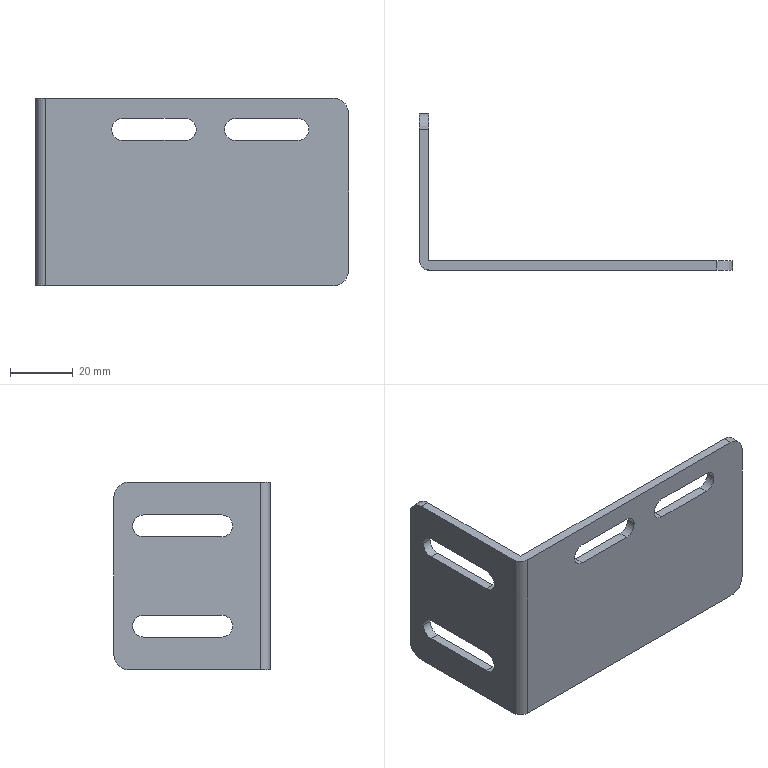Part | STEP file | X Travel Bracket 2 | 1 solid | 32 faces | box 100 x 50 x 60 mm | volume 23920 mm3 | cylinder 16 | plane 16 | commonest cylinder face diameters 7 x10 10 x4 0.2 x1 6.2 x1
STEP:
#1=CARTESIAN_POINT('',(-18.962,-0.4258,49.5));
#2=VERTEX_POINT('',#1);
#3=CARTESIAN_POINT('',(-18.962,3.074,46.));
#4=VERTEX_POINT('',#3);
#5=CARTESIAN_POINT('',(-18.962,-0.4258,46.));
#6=DIRECTION('',(-1.,0.,0.));
#7=DIRECTION('',(0.,1.,0.));
#8=AXIS2_PLACEMENT_3D('',#5,#6,#7);
#9=CIRCLE('',#8,3.5);
#10=EDGE_CURVE('',#2,#4,#9,.T.);
#11=ORIENTED_EDGE('',*,*,#10,.T.);
#12=CARTESIAN_POINT('',(-15.962,3.074,46.));
#13=VERTEX_POINT('',#12);
#14=CARTESIAN_POINT('',(-25.962,3.074,46.));
#15=DIRECTION('',(1.,0.,0.));
#16=VECTOR('',#15,1000.);
#17=LINE('',#14,#16);
#18=EDGE_CURVE('',#4,#13,#17,.T.);
#19=ORIENTED_EDGE('',*,*,#18,.T.);
#20=CARTESIAN_POINT('',(-15.962,-0.4258,49.5));
#21=VERTEX_POINT('',#20);
#22=CARTESIAN_POINT('',(-15.962,-0.4258,46.));
#23=DIRECTION('',(-1.,0.,0.));
#24=DIRECTION('',(0.,1.,0.));
#25=AXIS2_PLACEMENT_3D('',#22,#23,#24);
#26=CIRCLE('',#25,3.5);
#27=EDGE_CURVE('',#21,#13,#26,.T.);
#28=ORIENTED_EDGE('',*,*,#27,.F.);
#29=CARTESIAN_POINT('',(-25.962,-0.4258,49.5));
#30=DIRECTION('',(1.,0.,0.));
#31=VECTOR('',#30,1000.);
#32=LINE('',#29,#31);
#33=EDGE_CURVE('',#2,#21,#32,.T.);
#34=ORIENTED_EDGE('',*,*,#33,.F.);
#35=EDGE_LOOP('',(#11,#19,#28,#34));
#36=FACE_OUTER_BOUND('',#35,.T.);
#37=CARTESIAN_POINT('',(-25.962,-0.4258,46.));
#38=DIRECTION('',(1.,0.,0.));
#39=DIRECTION('',(0.,1.,0.));
#40=AXIS2_PLACEMENT_3D('',#37,#38,#39);
#41=CYLINDRICAL_SURFACE('',#40,3.5);
#42=ADVANCED_FACE('',(#36),#41,.F.);
#43=CARTESIAN_POINT('',(-18.962,-0.4258,17.5));
#44=VERTEX_POINT('',#43);
#45=CARTESIAN_POINT('',(-18.962,3.074,14.));
#46=VERTEX_POINT('',#45);
#47=CARTESIAN_POINT('',(-18.962,-0.4258,14.));
#48=DIRECTION('',(-1.,0.,0.));
#49=DIRECTION('',(0.,1.,0.));
#50=AXIS2_PLACEMENT_3D('',#47,#48,#49);
#51=CIRCLE('',#50,3.5);
#52=EDGE_CURVE('',#44,#46,#51,.T.);
#53=ORIENTED_EDGE('',*,*,#52,.T.);
#54=CARTESIAN_POINT('',(-15.962,3.074,14.));
#55=VERTEX_POINT('',#54);
#56=CARTESIAN_POINT('',(-25.962,3.074,14.));
#57=DIRECTION('',(1.,0.,0.));
#58=VECTOR('',#57,1000.);
#59=LINE('',#56,#58);
#60=EDGE_CURVE('',#46,#55,#59,.T.);
#61=ORIENTED_EDGE('',*,*,#60,.T.);
#62=CARTESIAN_POINT('',(-15.962,-0.4258,17.5));
#63=VERTEX_POINT('',#62);
#64=CARTESIAN_POINT('',(-15.962,-0.4258,14.));
#65=DIRECTION('',(-1.,0.,0.));
#66=DIRECTION('',(0.,1.,0.));
#67=AXIS2_PLACEMENT_3D('',#64,#65,#66);
#68=CIRCLE('',#67,3.5);
#69=EDGE_CURVE('',#63,#55,#68,.T.);
#70=ORIENTED_EDGE('',*,*,#69,.F.);
#71=CARTESIAN_POINT('',(-25.962,-0.4258,17.5));
#72=DIRECTION('',(1.,0.,0.));
#73=VECTOR('',#72,1000.);
#74=LINE('',#71,#73);
#75=EDGE_CURVE('',#44,#63,#74,.T.);
#76=ORIENTED_EDGE('',*,*,#75,.F.);
#77=EDGE_LOOP('',(#53,#61,#70,#76));
#78=FACE_OUTER_BOUND('',#77,.T.);
#79=CARTESIAN_POINT('',(-25.962,-0.4258,14.));
#80=DIRECTION('',(1.,0.,0.));
#81=DIRECTION('',(0.,1.,0.));
#82=AXIS2_PLACEMENT_3D('',#79,#80,#81);
#83=CYLINDRICAL_SURFACE('',#82,3.5);
#84=ADVANCED_FACE('',(#78),#83,.F.);
#85=CARTESIAN_POINT('',(81.038,-40.926,5.));
#86=VERTEX_POINT('',#85);
#87=CARTESIAN_POINT('',(76.038,-40.926,0.));
#88=VERTEX_POINT('',#87);
#89=CARTESIAN_POINT('',(76.038,-40.926,5.));
#90=DIRECTION('',(0.,1.,0.));
#91=DIRECTION('',(0.,0.,-1.));
#92=AXIS2_PLACEMENT_3D('',#89,#90,#91);
#93=CIRCLE('',#92,5.);
#94=EDGE_CURVE('',#86,#88,#93,.T.);
#95=ORIENTED_EDGE('',*,*,#94,.F.);
#96=CARTESIAN_POINT('',(81.038,-40.926,55.));
#97=VERTEX_POINT('',#96);
#98=CARTESIAN_POINT('',(81.038,-40.926,60.));
#99=DIRECTION('',(0.,0.,-1.));
#100=VECTOR('',#99,1000.);
#101=LINE('',#98,#100);
#102=EDGE_CURVE('',#97,#86,#101,.T.);
#103=ORIENTED_EDGE('',*,*,#102,.F.);
#104=CARTESIAN_POINT('',(76.038,-40.926,60.));
#105=VERTEX_POINT('',#104);
#106=CARTESIAN_POINT('',(76.038,-40.926,55.));
#107=DIRECTION('',(0.,1.,0.));
#108=DIRECTION('',(0.,0.,-1.));
#109=AXIS2_PLACEMENT_3D('',#106,#107,#108);
#110=CIRCLE('',#109,5.);
#111=EDGE_CURVE('',#105,#97,#110,.T.);
#112=ORIENTED_EDGE('',*,*,#111,.F.);
#113=CARTESIAN_POINT('',(-15.862,-40.926,60.));
#114=VERTEX_POINT('',#113);
#115=CARTESIAN_POINT('',(-18.962,-40.926,60.));
#116=DIRECTION('',(1.,0.,0.));
#117=VECTOR('',#116,1000.);
#118=LINE('',#115,#117);
#119=EDGE_CURVE('',#114,#105,#118,.T.);
#120=ORIENTED_EDGE('',*,*,#119,.F.);
#121=CARTESIAN_POINT('',(-15.862,-40.926,0.));
#122=VERTEX_POINT('',#121);
#123=CARTESIAN_POINT('',(-15.862,-40.926,60.));
#124=DIRECTION('',(0.,0.,1.));
#125=VECTOR('',#124,1000.);
#126=LINE('',#123,#125);
#127=EDGE_CURVE('',#122,#114,#126,.T.);
#128=ORIENTED_EDGE('',*,*,#127,.F.);
#129=CARTESIAN_POINT('',(-18.962,-40.926,0.));
#130=DIRECTION('',(-1.,0.,0.));
#131=VECTOR('',#130,1000.);
#132=LINE('',#129,#131);
#133=EDGE_CURVE('',#88,#122,#132,.T.);
#134=ORIENTED_EDGE('',*,*,#133,.F.);
#135=EDGE_LOOP('',(#95,#103,#112,#120,#128,#134));
#136=FACE_OUTER_BOUND('',#135,.T.);
#137=CARTESIAN_POINT('',(8.866,-40.926,53.5));
#138=VERTEX_POINT('',#137);
#139=CARTESIAN_POINT('',(8.866,-40.926,46.5));
#140=VERTEX_POINT('',#139);
#141=CARTESIAN_POINT('',(8.866,-40.926,50.));
#142=DIRECTION('',(0.,-1.,0.));
#143=DIRECTION('',(0.,0.,1.));
#144=AXIS2_PLACEMENT_3D('',#141,#142,#143);
#145=CIRCLE('',#144,3.5);
#146=EDGE_CURVE('',#138,#140,#145,.T.);
#147=ORIENTED_EDGE('',*,*,#146,.F.);
#148=CARTESIAN_POINT('',(28.866,-40.926,53.5));
#149=VERTEX_POINT('',#148);
#150=CARTESIAN_POINT('',(-18.962,-40.926,53.5));
#151=DIRECTION('',(-1.,0.,0.));
#152=VECTOR('',#151,1000.);
#153=LINE('',#150,#152);
#154=EDGE_CURVE('',#149,#138,#153,.T.);
#155=ORIENTED_EDGE('',*,*,#154,.F.);
#156=CARTESIAN_POINT('',(28.866,-40.926,46.5));
#157=VERTEX_POINT('',#156);
#158=CARTESIAN_POINT('',(28.866,-40.926,50.));
#159=DIRECTION('',(0.,-1.,0.));
#160=DIRECTION('',(0.,0.,1.));
#161=AXIS2_PLACEMENT_3D('',#158,#159,#160);
#162=CIRCLE('',#161,3.5);
#163=EDGE_CURVE('',#157,#149,#162,.T.);
#164=ORIENTED_EDGE('',*,*,#163,.F.);
#165=CARTESIAN_POINT('',(-18.962,-40.926,46.5));
#166=DIRECTION('',(1.,0.,0.));
#167=VECTOR('',#166,1000.);
#168=LINE('',#165,#167);
#169=EDGE_CURVE('',#140,#157,#168,.T.);
#170=ORIENTED_EDGE('',*,*,#169,.F.);
#171=EDGE_LOOP('',(#147,#155,#164,#170));
#172=FACE_BOUND('',#171,.T.);
#173=CARTESIAN_POINT('',(44.866,-40.926,53.5));
#174=VERTEX_POINT('',#173);
#175=CARTESIAN_POINT('',(44.866,-40.926,46.5));
#176=VERTEX_POINT('',#175);
#177=CARTESIAN_POINT('',(44.866,-40.926,50.));
#178=DIRECTION('',(0.,-1.,0.));
#179=DIRECTION('',(0.,0.,1.));
#180=AXIS2_PLACEMENT_3D('',#177,#178,#179);
#181=CIRCLE('',#180,3.5);
#182=EDGE_CURVE('',#174,#176,#181,.T.);
#183=ORIENTED_EDGE('',*,*,#182,.F.);
#184=CARTESIAN_POINT('',(64.866,-40.926,53.5));
#185=VERTEX_POINT('',#184);
#186=CARTESIAN_POINT('',(-18.962,-40.926,53.5));
#187=DIRECTION('',(-1.,0.,0.));
#188=VECTOR('',#187,1000.);
#189=LINE('',#186,#188);
#190=EDGE_CURVE('',#185,#174,#189,.T.);
#191=ORIENTED_EDGE('',*,*,#190,.F.);
#192=CARTESIAN_POINT('',(64.866,-40.926,46.5));
#193=VERTEX_POINT('',#192);
#194=CARTESIAN_POINT('',(64.866,-40.926,50.));
#195=DIRECTION('',(0.,-1.,0.));
#196=DIRECTION('',(0.,0.,1.));
#197=AXIS2_PLACEMENT_3D('',#194,#195,#196);
#198=CIRCLE('',#197,3.5);
#199=EDGE_CURVE('',#193,#185,#198,.T.);
#200=ORIENTED_EDGE('',*,*,#199,.F.);
#201=CARTESIAN_POINT('',(-18.962,-40.926,46.5));
#202=DIRECTION('',(1.,0.,0.));
#203=VECTOR('',#202,1000.);
#204=LINE('',#201,#203);
#205=EDGE_CURVE('',#176,#193,#204,.T.);
#206=ORIENTED_EDGE('',*,*,#205,.F.);
#207=EDGE_LOOP('',(#183,#191,#200,#206));
#208=FACE_BOUND('',#207,.T.);
#209=CARTESIAN_POINT('',(-18.962,-40.926,60.));
#210=DIRECTION('',(0.,1.,0.));
#211=DIRECTION('',(0.,0.,1.));
#212=AXIS2_PLACEMENT_3D('',#209,#210,#211);
#213=PLANE('',#212);
#214=ADVANCED_FACE('',(#136,#172,#208),#213,.F.);
#215=ORIENTED_EDGE('',*,*,#133,.T.);
#216=CARTESIAN_POINT('',(-18.962,-37.826,0.));
#217=VERTEX_POINT('',#216);
#218=CARTESIAN_POINT('',(-15.862,-37.826,0.));
#219=DIRECTION('',(0.,0.,1.));
#220=DIRECTION('',(-1.,0.,0.));
#221=AXIS2_PLACEMENT_3D('',#218,#219,#220);
#222=CIRCLE('',#221,3.1);
#223=EDGE_CURVE('',#217,#122,#222,.T.);
#224=ORIENTED_EDGE('',*,*,#223,.F.);
#225=CARTESIAN_POINT('',(-18.962,4.074,0.));
#226=VERTEX_POINT('',#225);
#227=CARTESIAN_POINT('',(-18.962,9.074,0.));
#228=DIRECTION('',(0.,1.,0.));
#229=VECTOR('',#228,1000.);
#230=LINE('',#227,#229);
#231=EDGE_CURVE('',#217,#226,#230,.T.);
#232=ORIENTED_EDGE('',*,*,#231,.T.);
#233=CARTESIAN_POINT('',(-15.962,4.074,0.));
#234=VERTEX_POINT('',#233);
#235=CARTESIAN_POINT('',(-15.862,4.074,0.));
#236=DIRECTION('',(-1.,0.,0.));
#237=VECTOR('',#236,1000.);
#238=LINE('',#235,#237);
#239=EDGE_CURVE('',#234,#226,#238,.T.);
#240=ORIENTED_EDGE('',*,*,#239,.F.);
#241=CARTESIAN_POINT('',(-15.962,-37.826,0.));
#242=VERTEX_POINT('',#241);
#243=CARTESIAN_POINT('',(-15.962,-37.826,0.));
#244=DIRECTION('',(0.,1.,0.));
#245=VECTOR('',#244,1000.);
#246=LINE('',#243,#245);
#247=EDGE_CURVE('',#242,#234,#246,.T.);
#248=ORIENTED_EDGE('',*,*,#247,.F.);
#249=CARTESIAN_POINT('',(-15.862,-37.926,0.));
#250=VERTEX_POINT('',#249);
#251=CARTESIAN_POINT('',(-15.862,-37.826,0.));
#252=DIRECTION('',(0.,0.,1.));
#253=DIRECTION('',(-1.,0.,0.));
#254=AXIS2_PLACEMENT_3D('',#251,#252,#253);
#255=CIRCLE('',#254,0.1);
#256=EDGE_CURVE('',#242,#250,#255,.T.);
#257=ORIENTED_EDGE('',*,*,#256,.T.);
#258=CARTESIAN_POINT('',(76.038,-37.926,0.));
#259=VERTEX_POINT('',#258);
#260=CARTESIAN_POINT('',(-15.962,-37.926,0.));
#261=DIRECTION('',(1.,0.,0.));
#262=VECTOR('',#261,1000.);
#263=LINE('',#260,#262);
#264=EDGE_CURVE('',#250,#259,#263,.T.);
#265=ORIENTED_EDGE('',*,*,#264,.T.);
#266=CARTESIAN_POINT('',(76.038,-37.826,0.));
#267=DIRECTION('',(0.,-1.,0.));
#268=VECTOR('',#267,1000.);
#269=LINE('',#266,#268);
#270=EDGE_CURVE('',#259,#88,#269,.T.);
#271=ORIENTED_EDGE('',*,*,#270,.T.);
#272=EDGE_LOOP('',(#215,#224,#232,#240,#248,#257,#265,#271));
#273=FACE_OUTER_BOUND('',#272,.T.);
#274=CARTESIAN_POINT('',(-15.962,-37.826,0.));
#275=DIRECTION('',(0.,0.,-1.));
#276=DIRECTION('',(-1.,0.,0.));
#277=AXIS2_PLACEMENT_3D('',#274,#275,#276);
#278=PLANE('',#277);
#279=ADVANCED_FACE('',(#273),#278,.T.);
#280=ORIENTED_EDGE('',*,*,#94,.T.);
#281=ORIENTED_EDGE('',*,*,#270,.F.);
#282=CARTESIAN_POINT('',(81.038,-37.926,5.));
#283=VERTEX_POINT('',#282);
#284=CARTESIAN_POINT('',(76.038,-37.926,5.));
#285=DIRECTION('',(0.,-1.,0.));
#286=DIRECTION('',(0.,0.,-1.));
#287=AXIS2_PLACEMENT_3D('',#284,#285,#286);
#288=CIRCLE('',#287,5.);
#289=EDGE_CURVE('',#259,#283,#288,.T.);
#290=ORIENTED_EDGE('',*,*,#289,.T.);
#291=CARTESIAN_POINT('',(81.038,-37.826,5.));
#292=DIRECTION('',(0.,-1.,0.));
#293=VECTOR('',#292,1000.);
#294=LINE('',#291,#293);
#295=EDGE_CURVE('',#283,#86,#294,.T.);
#296=ORIENTED_EDGE('',*,*,#295,.T.);
#297=EDGE_LOOP('',(#280,#281,#290,#296));
#298=FACE_OUTER_BOUND('',#297,.T.);
#299=CARTESIAN_POINT('',(76.038,-37.826,5.));
#300=DIRECTION('',(0.,-1.,0.));
#301=DIRECTION('',(0.,0.,-1.));
#302=AXIS2_PLACEMENT_3D('',#299,#300,#301);
#303=CYLINDRICAL_SURFACE('',#302,5.);
#304=ADVANCED_FACE('',(#298),#303,.T.);
#305=CARTESIAN_POINT('',(81.038,-37.926,55.));
#306=VERTEX_POINT('',#305);
#307=CARTESIAN_POINT('',(81.038,-37.926,60.));
#308=DIRECTION('',(0.,0.,1.));
#309=VECTOR('',#308,1000.);
#310=LINE('',#307,#309);
#311=EDGE_CURVE('',#283,#306,#310,.T.);
#312=ORIENTED_EDGE('',*,*,#311,.T.);
#313=CARTESIAN_POINT('',(81.038,-37.926,55.));
#314=DIRECTION('',(0.,-1.,0.));
#315=VECTOR('',#314,1000.);
#316=LINE('',#313,#315);
#317=EDGE_CURVE('',#306,#97,#316,.T.);
#318=ORIENTED_EDGE('',*,*,#317,.T.);
#319=ORIENTED_EDGE('',*,*,#102,.T.);
#320=ORIENTED_EDGE('',*,*,#295,.F.);
#321=EDGE_LOOP('',(#312,#318,#319,#320));
#322=FACE_OUTER_BOUND('',#321,.T.);
#323=CARTESIAN_POINT('',(81.038,-37.926,60.));
#324=DIRECTION('',(1.,0.,0.));
#325=DIRECTION('',(0.,0.,-1.));
#326=AXIS2_PLACEMENT_3D('',#323,#324,#325);
#327=PLANE('',#326);
#328=ADVANCED_FACE('',(#322),#327,.T.);
#329=ORIENTED_EDGE('',*,*,#111,.T.);
#330=ORIENTED_EDGE('',*,*,#317,.F.);
#331=CARTESIAN_POINT('',(76.038,-37.926,60.));
#332=VERTEX_POINT('',#331);
#333=CARTESIAN_POINT('',(76.038,-37.926,55.));
#334=DIRECTION('',(0.,-1.,0.));
#335=DIRECTION('',(0.,0.,-1.));
#336=AXIS2_PLACEMENT_3D('',#333,#334,#335);
#337=CIRCLE('',#336,5.);
#338=EDGE_CURVE('',#306,#332,#337,.T.);
#339=ORIENTED_EDGE('',*,*,#338,.T.);
#340=CARTESIAN_POINT('',(76.038,-37.926,60.));
#341=DIRECTION('',(0.,-1.,0.));
#342=VECTOR('',#341,1000.);
#343=LINE('',#340,#342);
#344=EDGE_CURVE('',#332,#105,#343,.T.);
#345=ORIENTED_EDGE('',*,*,#344,.T.);
#346=EDGE_LOOP('',(#329,#330,#339,#345));
#347=FACE_OUTER_BOUND('',#346,.T.);
#348=CARTESIAN_POINT('',(76.038,-37.926,55.));
#349=DIRECTION('',(0.,-1.,0.));
#350=DIRECTION('',(0.,0.,-1.));
#351=AXIS2_PLACEMENT_3D('',#348,#349,#350);
#352=CYLINDRICAL_SURFACE('',#351,5.);
#353=ADVANCED_FACE('',(#347),#352,.T.);
#354=CARTESIAN_POINT('',(-15.862,-37.926,60.));
#355=VERTEX_POINT('',#354);
#356=CARTESIAN_POINT('',(-15.862,-37.926,60.));
#357=DIRECTION('',(-1.,0.,0.));
#358=VECTOR('',#357,1000.);
#359=LINE('',#356,#358);
#360=EDGE_CURVE('',#332,#355,#359,.T.);
#361=ORIENTED_EDGE('',*,*,#360,.T.);
#362=CARTESIAN_POINT('',(-15.962,-37.826,60.));
#363=VERTEX_POINT('',#362);
#364=CARTESIAN_POINT('',(-15.862,-37.826,60.));
#365=DIRECTION('',(0.,0.,-1.));
#366=DIRECTION('',(-1.,0.,0.));
#367=AXIS2_PLACEMENT_3D('',#364,#365,#366);
#368=CIRCLE('',#367,0.1);
#369=EDGE_CURVE('',#355,#363,#368,.T.);
#370=ORIENTED_EDGE('',*,*,#369,.T.);
#371=CARTESIAN_POINT('',(-15.962,4.074,60.));
#372=VERTEX_POINT('',#371);
#373=CARTESIAN_POINT('',(-15.962,-37.926,60.));
#374=DIRECTION('',(0.,1.,0.));
#375=VECTOR('',#374,1000.);
#376=LINE('',#373,#375);
#377=EDGE_CURVE('',#363,#372,#376,.T.);
#378=ORIENTED_EDGE('',*,*,#377,.T.);
#379=CARTESIAN_POINT('',(-18.962,4.074,60.));
#380=VERTEX_POINT('',#379);
#381=CARTESIAN_POINT('',(-15.862,4.074,60.));
#382=DIRECTION('',(-1.,0.,0.));
#383=VECTOR('',#382,1000.);
#384=LINE('',#381,#383);
#385=EDGE_CURVE('',#372,#380,#384,.T.);
#386=ORIENTED_EDGE('',*,*,#385,.T.);
#387=CARTESIAN_POINT('',(-18.962,-37.826,60.));
#388=VERTEX_POINT('',#387);
#389=CARTESIAN_POINT('',(-18.962,9.074,60.));
#390=DIRECTION('',(0.,-1.,0.));
#391=VECTOR('',#390,1000.);
#392=LINE('',#389,#391);
#393=EDGE_CURVE('',#380,#388,#392,.T.);
#394=ORIENTED_EDGE('',*,*,#393,.T.);
#395=CARTESIAN_POINT('',(-15.862,-37.826,60.));
#396=DIRECTION('',(0.,0.,-1.));
#397=DIRECTION('',(-1.,0.,0.));
#398=AXIS2_PLACEMENT_3D('',#395,#396,#397);
#399=CIRCLE('',#398,3.1);
#400=EDGE_CURVE('',#114,#388,#399,.T.);
#401=ORIENTED_EDGE('',*,*,#400,.F.);
#402=ORIENTED_EDGE('',*,*,#119,.T.);
#403=ORIENTED_EDGE('',*,*,#344,.F.);
#404=EDGE_LOOP('',(#361,#370,#378,#386,#394,#401,#402,#403));
#405=FACE_OUTER_BOUND('',#404,.T.);
#406=CARTESIAN_POINT('',(-15.862,-37.826,60.));
#407=DIRECTION('',(0.,0.,1.));
#408=DIRECTION('',(1.,0.,0.));
#409=AXIS2_PLACEMENT_3D('',#406,#407,#408);
#410=PLANE('',#409);
#411=ADVANCED_FACE('',(#405),#410,.T.);
#412=ORIENTED_EDGE('',*,*,#400,.T.);
#413=CARTESIAN_POINT('',(-18.962,-37.826,60.));
#414=DIRECTION('',(0.,0.,-1.));
#415=VECTOR('',#414,1000.);
#416=LINE('',#413,#415);
#417=EDGE_CURVE('',#388,#217,#416,.T.);
#418=ORIENTED_EDGE('',*,*,#417,.T.);
#419=ORIENTED_EDGE('',*,*,#223,.T.);
#420=ORIENTED_EDGE('',*,*,#127,.T.);
#421=EDGE_LOOP('',(#412,#418,#419,#420));
#422=FACE_OUTER_BOUND('',#421,.T.);
#423=CARTESIAN_POINT('',(-15.862,-37.826,60.));
#424=DIRECTION('',(0.,0.,-1.));
#425=DIRECTION('',(-1.,0.,0.));
#426=AXIS2_PLACEMENT_3D('',#423,#424,#425);
#427=CYLINDRICAL_SURFACE('',#426,3.1);
#428=ADVANCED_FACE('',(#422),#427,.T.);
#429=CARTESIAN_POINT('',(8.866,-37.926,46.5));
#430=VERTEX_POINT('',#429);
#431=CARTESIAN_POINT('',(28.866,-37.926,46.5));
#432=VERTEX_POINT('',#431);
#433=CARTESIAN_POINT('',(8.866,-37.926,46.5));
#434=DIRECTION('',(1.,0.,0.));
#435=VECTOR('',#434,1000.);
#436=LINE('',#433,#435);
#437=EDGE_CURVE('',#430,#432,#436,.T.);
#438=ORIENTED_EDGE('',*,*,#437,.F.);
#439=CARTESIAN_POINT('',(8.866,-47.926,46.5));
#440=DIRECTION('',(0.,1.,0.));
#441=VECTOR('',#440,1000.);
#442=LINE('',#439,#441);
#443=EDGE_CURVE('',#140,#430,#442,.T.);
#444=ORIENTED_EDGE('',*,*,#443,.F.);
#445=ORIENTED_EDGE('',*,*,#169,.T.);
#446=CARTESIAN_POINT('',(28.866,-47.926,46.5));
#447=DIRECTION('',(0.,-1.,0.));
#448=VECTOR('',#447,1000.);
#449=LINE('',#446,#448);
#450=EDGE_CURVE('',#432,#157,#449,.T.);
#451=ORIENTED_EDGE('',*,*,#450,.F.);
#452=EDGE_LOOP('',(#438,#444,#445,#451));
#453=FACE_OUTER_BOUND('',#452,.T.);
#454=CARTESIAN_POINT('',(8.866,-47.926,46.5));
#455=DIRECTION('',(0.,0.,-1.));
#456=DIRECTION('',(-1.,0.,0.));
#457=AXIS2_PLACEMENT_3D('',#454,#455,#456);
#458=PLANE('',#457);
#459=ADVANCED_FACE('',(#453),#458,.F.);
#460=CARTESIAN_POINT('',(8.866,-37.926,53.5));
#461=VERTEX_POINT('',#460);
#462=CARTESIAN_POINT('',(8.866,-37.926,50.));
#463=DIRECTION('',(0.,-1.,0.));
#464=DIRECTION('',(0.,0.,1.));
#465=AXIS2_PLACEMENT_3D('',#462,#463,#464);
#466=CIRCLE('',#465,3.5);
#467=EDGE_CURVE('',#461,#430,#466,.T.);
#468=ORIENTED_EDGE('',*,*,#467,.F.);
#469=CARTESIAN_POINT('',(8.866,-47.926,53.5));
#470=DIRECTION('',(0.,1.,0.));
#471=VECTOR('',#470,1000.);
#472=LINE('',#469,#471);
#473=EDGE_CURVE('',#138,#461,#472,.T.);
#474=ORIENTED_EDGE('',*,*,#473,.F.);
#475=ORIENTED_EDGE('',*,*,#146,.T.);
#476=ORIENTED_EDGE('',*,*,#443,.T.);
#477=EDGE_LOOP('',(#468,#474,#475,#476));
#478=FACE_OUTER_BOUND('',#477,.T.);
#479=CARTESIAN_POINT('',(8.866,-47.926,50.));
#480=DIRECTION('',(0.,1.,0.));
#481=DIRECTION('',(0.,0.,1.));
#482=AXIS2_PLACEMENT_3D('',#479,#480,#481);
#483=CYLINDRICAL_SURFACE('',#482,3.5);
#484=ADVANCED_FACE('',(#478),#483,.F.);
#485=CARTESIAN_POINT('',(28.866,-37.926,53.5));
#486=VERTEX_POINT('',#485);
#487=CARTESIAN_POINT('',(8.866,-37.926,53.5));
#488=DIRECTION('',(-1.,0.,0.));
#489=VECTOR('',#488,1000.);
#490=LINE('',#487,#489);
#491=EDGE_CURVE('',#486,#461,#490,.T.);
#492=ORIENTED_EDGE('',*,*,#491,.F.);
#493=CARTESIAN_POINT('',(28.866,-47.926,53.5));
#494=DIRECTION('',(0.,1.,0.));
#495=VECTOR('',#494,1000.);
#496=LINE('',#493,#495);
#497=EDGE_CURVE('',#149,#486,#496,.T.);
#498=ORIENTED_EDGE('',*,*,#497,.F.);
#499=ORIENTED_EDGE('',*,*,#154,.T.);
#500=ORIENTED_EDGE('',*,*,#473,.T.);
#501=EDGE_LOOP('',(#492,#498,#499,#500));
#502=FACE_OUTER_BOUND('',#501,.T.);
#503=CARTESIAN_POINT('',(8.866,-47.926,53.5));
#504=DIRECTION('',(0.,0.,1.));
#505=DIRECTION('',(1.,0.,0.));
#506=AXIS2_PLACEMENT_3D('',#503,#504,#505);
#507=PLANE('',#506);
#508=ADVANCED_FACE('',(#502),#507,.F.);
#509=CARTESIAN_POINT('',(28.866,-37.926,50.));
#510=DIRECTION('',(0.,-1.,0.));
#511=DIRECTION('',(0.,0.,1.));
#512=AXIS2_PLACEMENT_3D('',#509,#510,#511);
#513=CIRCLE('',#512,3.5);
#514=EDGE_CURVE('',#432,#486,#513,.T.);
#515=ORIENTED_EDGE('',*,*,#514,.F.);
#516=ORIENTED_EDGE('',*,*,#450,.T.);
#517=ORIENTED_EDGE('',*,*,#163,.T.);
#518=ORIENTED_EDGE('',*,*,#497,.T.);
#519=EDGE_LOOP('',(#515,#516,#517,#518));
#520=FACE_OUTER_BOUND('',#519,.T.);
#521=CARTESIAN_POINT('',(28.866,-47.926,50.));
#522=DIRECTION('',(0.,1.,0.));
#523=DIRECTION('',(0.,0.,1.));
#524=AXIS2_PLACEMENT_3D('',#521,#522,#523);
#525=CYLINDRICAL_SURFACE('',#524,3.5);
#526=ADVANCED_FACE('',(#520),#525,.F.);
#527=CARTESIAN_POINT('',(44.866,-37.926,46.5));
#528=VERTEX_POINT('',#527);
#529=CARTESIAN_POINT('',(64.866,-37.926,46.5));
#530=VERTEX_POINT('',#529);
#531=CARTESIAN_POINT('',(44.866,-37.926,46.5));
#532=DIRECTION('',(1.,0.,0.));
#533=VECTOR('',#532,1000.);
#534=LINE('',#531,#533);
#535=EDGE_CURVE('',#528,#530,#534,.T.);
#536=ORIENTED_EDGE('',*,*,#535,.F.);
#537=CARTESIAN_POINT('',(44.866,-47.926,46.5));
#538=DIRECTION('',(0.,1.,0.));
#539=VECTOR('',#538,1000.);
#540=LINE('',#537,#539);
#541=EDGE_CURVE('',#176,#528,#540,.T.);
#542=ORIENTED_EDGE('',*,*,#541,.F.);
#543=ORIENTED_EDGE('',*,*,#205,.T.);
#544=CARTESIAN_POINT('',(64.866,-47.926,46.5));
#545=DIRECTION('',(0.,-1.,0.));
#546=VECTOR('',#545,1000.);
#547=LINE('',#544,#546);
#548=EDGE_CURVE('',#530,#193,#547,.T.);
#549=ORIENTED_EDGE('',*,*,#548,.F.);
#550=EDGE_LOOP('',(#536,#542,#543,#549));
#551=FACE_OUTER_BOUND('',#550,.T.);
#552=CARTESIAN_POINT('',(44.866,-47.926,46.5));
#553=DIRECTION('',(0.,0.,-1.));
#554=DIRECTION('',(-1.,0.,0.));
#555=AXIS2_PLACEMENT_3D('',#552,#553,#554);
#556=PLANE('',#555);
#557=ADVANCED_FACE('',(#551),#556,.F.);
#558=CARTESIAN_POINT('',(44.866,-37.926,53.5));
#559=VERTEX_POINT('',#558);
#560=CARTESIAN_POINT('',(44.866,-37.926,50.));
#561=DIRECTION('',(0.,-1.,0.));
#562=DIRECTION('',(0.,0.,1.));
#563=AXIS2_PLACEMENT_3D('',#560,#561,#562);
#564=CIRCLE('',#563,3.5);
#565=EDGE_CURVE('',#559,#528,#564,.T.);
#566=ORIENTED_EDGE('',*,*,#565,.F.);
#567=CARTESIAN_POINT('',(44.866,-47.926,53.5));
#568=DIRECTION('',(0.,1.,0.));
#569=VECTOR('',#568,1000.);
#570=LINE('',#567,#569);
#571=EDGE_CURVE('',#174,#559,#570,.T.);
#572=ORIENTED_EDGE('',*,*,#571,.F.);
#573=ORIENTED_EDGE('',*,*,#182,.T.);
#574=ORIENTED_EDGE('',*,*,#541,.T.);
#575=EDGE_LOOP('',(#566,#572,#573,#574));
#576=FACE_OUTER_BOUND('',#575,.T.);
#577=CARTESIAN_POINT('',(44.866,-47.926,50.));
#578=DIRECTION('',(0.,1.,0.));
#579=DIRECTION('',(0.,0.,1.));
#580=AXIS2_PLACEMENT_3D('',#577,#578,#579);
#581=CYLINDRICAL_SURFACE('',#580,3.5);
#582=ADVANCED_FACE('',(#576),#581,.F.);
#583=CARTESIAN_POINT('',(64.866,-37.926,53.5));
#584=VERTEX_POINT('',#583);
#585=CARTESIAN_POINT('',(44.866,-37.926,53.5));
#586=DIRECTION('',(-1.,0.,0.));
#587=VECTOR('',#586,1000.);
#588=LINE('',#585,#587);
#589=EDGE_CURVE('',#584,#559,#588,.T.);
#590=ORIENTED_EDGE('',*,*,#589,.F.);
#591=CARTESIAN_POINT('',(64.866,-47.926,53.5));
#592=DIRECTION('',(0.,1.,0.));
#593=VECTOR('',#592,1000.);
#594=LINE('',#591,#593);
#595=EDGE_CURVE('',#185,#584,#594,.T.);
#596=ORIENTED_EDGE('',*,*,#595,.F.);
#597=ORIENTED_EDGE('',*,*,#190,.T.);
#598=ORIENTED_EDGE('',*,*,#571,.T.);
#599=EDGE_LOOP('',(#590,#596,#597,#598));
#600=FACE_OUTER_BOUND('',#599,.T.);
#601=CARTESIAN_POINT('',(44.866,-47.926,53.5));
#602=DIRECTION('',(0.,0.,1.));
#603=DIRECTION('',(1.,0.,0.));
#604=AXIS2_PLACEMENT_3D('',#601,#602,#603);
#605=PLANE('',#604);
#606=ADVANCED_FACE('',(#600),#605,.F.);
#607=CARTESIAN_POINT('',(64.866,-37.926,50.));
#608=DIRECTION('',(0.,-1.,0.));
#609=DIRECTION('',(0.,0.,1.));
#610=AXIS2_PLACEMENT_3D('',#607,#608,#609);
#611=CIRCLE('',#610,3.5);
#612=EDGE_CURVE('',#530,#584,#611,.T.);
#613=ORIENTED_EDGE('',*,*,#612,.F.);
#614=ORIENTED_EDGE('',*,*,#548,.T.);
#615=ORIENTED_EDGE('',*,*,#199,.T.);
#616=ORIENTED_EDGE('',*,*,#595,.T.);
#617=EDGE_LOOP('',(#613,#614,#615,#616));
#618=FACE_OUTER_BOUND('',#617,.T.);
#619=CARTESIAN_POINT('',(64.866,-47.926,50.));
#620=DIRECTION('',(0.,1.,0.));
#621=DIRECTION('',(0.,0.,1.));
#622=AXIS2_PLACEMENT_3D('',#619,#620,#621);
#623=CYLINDRICAL_SURFACE('',#622,3.5);
#624=ADVANCED_FACE('',(#618),#623,.F.);
#625=ORIENTED_EDGE('',*,*,#360,.F.);
#626=ORIENTED_EDGE('',*,*,#338,.F.);
#627=ORIENTED_EDGE('',*,*,#311,.F.);
#628=ORIENTED_EDGE('',*,*,#289,.F.);
#629=ORIENTED_EDGE('',*,*,#264,.F.);
#630=CARTESIAN_POINT('',(-15.862,-37.926,60.));
#631=DIRECTION('',(0.,0.,1.));
#632=VECTOR('',#631,1000.);
#633=LINE('',#630,#632);
#634=EDGE_CURVE('',#250,#355,#633,.T.);
#635=ORIENTED_EDGE('',*,*,#634,.T.);
#636=EDGE_LOOP('',(#625,#626,#627,#628,#629,#635));
#637=FACE_OUTER_BOUND('',#636,.T.);
#638=ORIENTED_EDGE('',*,*,#514,.T.);
#639=ORIENTED_EDGE('',*,*,#491,.T.);
#640=ORIENTED_EDGE('',*,*,#467,.T.);
#641=ORIENTED_EDGE('',*,*,#437,.T.);
#642=EDGE_LOOP('',(#638,#639,#640,#641));
#643=FACE_BOUND('',#642,.T.);
#644=ORIENTED_EDGE('',*,*,#612,.T.);
#645=ORIENTED_EDGE('',*,*,#589,.T.);
#646=ORIENTED_EDGE('',*,*,#565,.T.);
#647=ORIENTED_EDGE('',*,*,#535,.T.);
#648=EDGE_LOOP('',(#644,#645,#646,#647));
#649=FACE_BOUND('',#648,.T.);
#650=CARTESIAN_POINT('',(-18.962,-37.926,60.));
#651=DIRECTION('',(0.,1.,0.));
#652=DIRECTION('',(0.,0.,1.));
#653=AXIS2_PLACEMENT_3D('',#650,#651,#652);
#654=PLANE('',#653);
#655=ADVANCED_FACE('',(#637,#643,#649),#654,.T.);
#656=CARTESIAN_POINT('',(-18.962,9.074,5.));
#657=VERTEX_POINT('',#656);
#658=CARTESIAN_POINT('',(-18.962,4.074,5.));
#659=DIRECTION('',(1.,0.,0.));
#660=DIRECTION('',(0.,0.,1.));
#661=AXIS2_PLACEMENT_3D('',#658,#659,#660);
#662=CIRCLE('',#661,5.);
#663=EDGE_CURVE('',#226,#657,#662,.T.);
#664=ORIENTED_EDGE('',*,*,#663,.F.);
#665=ORIENTED_EDGE('',*,*,#231,.F.);
#666=ORIENTED_EDGE('',*,*,#417,.F.);
#667=ORIENTED_EDGE('',*,*,#393,.F.);
#668=CARTESIAN_POINT('',(-18.962,9.074,55.));
#669=VERTEX_POINT('',#668);
#670=CARTESIAN_POINT('',(-18.962,4.074,55.));
#671=DIRECTION('',(1.,0.,0.));
#672=DIRECTION('',(0.,0.,-1.));
#673=AXIS2_PLACEMENT_3D('',#670,#671,#672);
#674=CIRCLE('',#673,5.);
#675=EDGE_CURVE('',#669,#380,#674,.T.);
#676=ORIENTED_EDGE('',*,*,#675,.F.);
#677=CARTESIAN_POINT('',(-18.962,9.074,60.));
#678=DIRECTION('',(0.,0.,1.));
#679=VECTOR('',#678,1000.);
#680=LINE('',#677,#679);
#681=EDGE_CURVE('',#657,#669,#680,.T.);
#682=ORIENTED_EDGE('',*,*,#681,.F.);
#683=EDGE_LOOP('',(#664,#665,#666,#667,#676,#682));
#684=FACE_OUTER_BOUND('',#683,.T.);
#685=ORIENTED_EDGE('',*,*,#10,.F.);
#686=CARTESIAN_POINT('',(-18.962,-25.426,49.5));
#687=VERTEX_POINT('',#686);
#688=CARTESIAN_POINT('',(-18.962,9.074,49.5));
#689=DIRECTION('',(0.,1.,0.));
#690=VECTOR('',#689,1000.);
#691=LINE('',#688,#690);
#692=EDGE_CURVE('',#687,#2,#691,.T.);
#693=ORIENTED_EDGE('',*,*,#692,.F.);
#694=CARTESIAN_POINT('',(-18.962,-25.426,42.5));
#695=VERTEX_POINT('',#694);
#696=CARTESIAN_POINT('',(-18.962,-25.426,46.));
#697=DIRECTION('',(-1.,0.,0.));
#698=DIRECTION('',(0.,1.,0.));
#699=AXIS2_PLACEMENT_3D('',#696,#697,#698);
#700=CIRCLE('',#699,3.5);
#701=EDGE_CURVE('',#695,#687,#700,.T.);
#702=ORIENTED_EDGE('',*,*,#701,.F.);
#703=CARTESIAN_POINT('',(-18.962,-0.4258,42.5));
#704=VERTEX_POINT('',#703);
#705=CARTESIAN_POINT('',(-18.962,9.074,42.5));
#706=DIRECTION('',(0.,-1.,0.));
#707=VECTOR('',#706,1000.);
#708=LINE('',#705,#707);
#709=EDGE_CURVE('',#704,#695,#708,.T.);
#710=ORIENTED_EDGE('',*,*,#709,.F.);
#711=CARTESIAN_POINT('',(-18.962,-0.4258,46.));
#712=DIRECTION('',(-1.,0.,0.));
#713=DIRECTION('',(0.,1.,0.));
#714=AXIS2_PLACEMENT_3D('',#711,#712,#713);
#715=CIRCLE('',#714,3.5);
#716=EDGE_CURVE('',#4,#704,#715,.T.);
#717=ORIENTED_EDGE('',*,*,#716,.F.);
#718=EDGE_LOOP('',(#685,#693,#702,#710,#717));
#719=FACE_BOUND('',#718,.T.);
#720=ORIENTED_EDGE('',*,*,#52,.F.);
#721=CARTESIAN_POINT('',(-18.962,-25.426,17.5));
#722=VERTEX_POINT('',#721);
#723=CARTESIAN_POINT('',(-18.962,9.074,17.5));
#724=DIRECTION('',(0.,1.,0.));
#725=VECTOR('',#724,1000.);
#726=LINE('',#723,#725);
#727=EDGE_CURVE('',#722,#44,#726,.T.);
#728=ORIENTED_EDGE('',*,*,#727,.F.);
#729=CARTESIAN_POINT('',(-18.962,-25.426,10.5));
#730=VERTEX_POINT('',#729);
#731=CARTESIAN_POINT('',(-18.962,-25.426,14.));
#732=DIRECTION('',(-1.,0.,0.));
#733=DIRECTION('',(0.,1.,0.));
#734=AXIS2_PLACEMENT_3D('',#731,#732,#733);
#735=CIRCLE('',#734,3.5);
#736=EDGE_CURVE('',#730,#722,#735,.T.);
#737=ORIENTED_EDGE('',*,*,#736,.F.);
#738=CARTESIAN_POINT('',(-18.962,-0.4258,10.5));
#739=VERTEX_POINT('',#738);
#740=CARTESIAN_POINT('',(-18.962,9.074,10.5));
#741=DIRECTION('',(0.,-1.,0.));
#742=VECTOR('',#741,1000.);
#743=LINE('',#740,#742);
#744=EDGE_CURVE('',#739,#730,#743,.T.);
#745=ORIENTED_EDGE('',*,*,#744,.F.);
#746=CARTESIAN_POINT('',(-18.962,-0.4258,14.));
#747=DIRECTION('',(-1.,0.,0.));
#748=DIRECTION('',(0.,1.,0.));
#749=AXIS2_PLACEMENT_3D('',#746,#747,#748);
#750=CIRCLE('',#749,3.5);
#751=EDGE_CURVE('',#46,#739,#750,.T.);
#752=ORIENTED_EDGE('',*,*,#751,.F.);
#753=EDGE_LOOP('',(#720,#728,#737,#745,#752));
#754=FACE_BOUND('',#753,.T.);
#755=CARTESIAN_POINT('',(-18.962,9.074,60.));
#756=DIRECTION('',(1.,0.,0.));
#757=DIRECTION('',(0.,1.,0.));
#758=AXIS2_PLACEMENT_3D('',#755,#756,#757);
#759=PLANE('',#758);
#760=ADVANCED_FACE('',(#684,#719,#754),#759,.F.);
#761=CARTESIAN_POINT('',(-15.962,-37.826,60.));
#762=DIRECTION('',(0.,0.,-1.));
#763=VECTOR('',#762,1000.);
#764=LINE('',#761,#763);
#765=EDGE_CURVE('',#363,#242,#764,.T.);
#766=ORIENTED_EDGE('',*,*,#765,.F.);
#767=ORIENTED_EDGE('',*,*,#369,.F.);
#768=ORIENTED_EDGE('',*,*,#634,.F.);
#769=ORIENTED_EDGE('',*,*,#256,.F.);
#770=EDGE_LOOP('',(#766,#767,#768,#769));
#771=FACE_OUTER_BOUND('',#770,.T.);
#772=CARTESIAN_POINT('',(-15.862,-37.826,60.));
#773=DIRECTION('',(0.,0.,-1.));
#774=DIRECTION('',(-1.,0.,0.));
#775=AXIS2_PLACEMENT_3D('',#772,#773,#774);
#776=CYLINDRICAL_SURFACE('',#775,0.1);
#777=ADVANCED_FACE('',(#771),#776,.F.);
#778=ORIENTED_EDGE('',*,*,#681,.T.);
#779=CARTESIAN_POINT('',(-15.962,9.074,55.));
#780=VERTEX_POINT('',#779);
#781=CARTESIAN_POINT('',(-18.962,9.074,55.));
#782=DIRECTION('',(1.,0.,0.));
#783=VECTOR('',#782,1000.);
#784=LINE('',#781,#783);
#785=EDGE_CURVE('',#669,#780,#784,.T.);
#786=ORIENTED_EDGE('',*,*,#785,.T.);
#787=CARTESIAN_POINT('',(-15.962,9.074,5.));
#788=VERTEX_POINT('',#787);
#789=CARTESIAN_POINT('',(-15.962,9.074,60.));
#790=DIRECTION('',(0.,0.,-1.));
#791=VECTOR('',#790,1000.);
#792=LINE('',#789,#791);
#793=EDGE_CURVE('',#780,#788,#792,.T.);
#794=ORIENTED_EDGE('',*,*,#793,.T.);
#795=CARTESIAN_POINT('',(-18.962,9.074,5.));
#796=DIRECTION('',(-1.,0.,0.));
#797=VECTOR('',#796,1000.);
#798=LINE('',#795,#797);
#799=EDGE_CURVE('',#788,#657,#798,.T.);
#800=ORIENTED_EDGE('',*,*,#799,.T.);
#801=EDGE_LOOP('',(#778,#786,#794,#800));
#802=FACE_OUTER_BOUND('',#801,.T.);
#803=CARTESIAN_POINT('',(-18.962,9.074,60.));
#804=DIRECTION('',(0.,1.,0.));
#805=DIRECTION('',(0.,0.,1.));
#806=AXIS2_PLACEMENT_3D('',#803,#804,#805);
#807=PLANE('',#806);
#808=ADVANCED_FACE('',(#802),#807,.T.);
#809=CARTESIAN_POINT('',(-15.962,4.074,5.));
#810=DIRECTION('',(-1.,0.,0.));
#811=DIRECTION('',(0.,0.,1.));
#812=AXIS2_PLACEMENT_3D('',#809,#810,#811);
#813=CIRCLE('',#812,5.);
#814=EDGE_CURVE('',#788,#234,#813,.T.);
#815=ORIENTED_EDGE('',*,*,#814,.T.);
#816=ORIENTED_EDGE('',*,*,#239,.T.);
#817=ORIENTED_EDGE('',*,*,#663,.T.);
#818=ORIENTED_EDGE('',*,*,#799,.F.);
#819=EDGE_LOOP('',(#815,#816,#817,#818));
#820=FACE_OUTER_BOUND('',#819,.T.);
#821=CARTESIAN_POINT('',(-15.862,4.074,5.));
#822=DIRECTION('',(-1.,0.,0.));
#823=DIRECTION('',(0.,0.,1.));
#824=AXIS2_PLACEMENT_3D('',#821,#822,#823);
#825=CYLINDRICAL_SURFACE('',#824,5.);
#826=ADVANCED_FACE('',(#820),#825,.T.);
#827=CARTESIAN_POINT('',(-15.962,4.074,55.));
#828=DIRECTION('',(-1.,0.,0.));
#829=DIRECTION('',(0.,0.,-1.));
#830=AXIS2_PLACEMENT_3D('',#827,#828,#829);
#831=CIRCLE('',#830,5.);
#832=EDGE_CURVE('',#372,#780,#831,.T.);
#833=ORIENTED_EDGE('',*,*,#832,.T.);
#834=ORIENTED_EDGE('',*,*,#785,.F.);
#835=ORIENTED_EDGE('',*,*,#675,.T.);
#836=ORIENTED_EDGE('',*,*,#385,.F.);
#837=EDGE_LOOP('',(#833,#834,#835,#836));
#838=FACE_OUTER_BOUND('',#837,.T.);
#839=CARTESIAN_POINT('',(-18.962,4.074,55.));
#840=DIRECTION('',(1.,0.,0.));
#841=DIRECTION('',(0.,0.,-1.));
#842=AXIS2_PLACEMENT_3D('',#839,#840,#841);
#843=CYLINDRICAL_SURFACE('',#842,5.);
#844=ADVANCED_FACE('',(#838),#843,.T.);
#845=CARTESIAN_POINT('',(-15.962,-0.4258,42.5));
#846=VERTEX_POINT('',#845);
#847=CARTESIAN_POINT('',(-15.962,-25.426,42.5));
#848=VERTEX_POINT('',#847);
#849=CARTESIAN_POINT('',(-15.962,-0.4258,42.5));
#850=DIRECTION('',(0.,-1.,0.));
#851=VECTOR('',#850,1000.);
#852=LINE('',#849,#851);
#853=EDGE_CURVE('',#846,#848,#852,.T.);
#854=ORIENTED_EDGE('',*,*,#853,.F.);
#855=CARTESIAN_POINT('',(-25.962,-0.4258,42.5));
#856=DIRECTION('',(1.,0.,0.));
#857=VECTOR('',#856,1000.);
#858=LINE('',#855,#857);
#859=EDGE_CURVE('',#704,#846,#858,.T.);
#860=ORIENTED_EDGE('',*,*,#859,.F.);
#861=ORIENTED_EDGE('',*,*,#709,.T.);
#862=CARTESIAN_POINT('',(-25.962,-25.426,42.5));
#863=DIRECTION('',(-1.,0.,0.));
#864=VECTOR('',#863,1000.);
#865=LINE('',#862,#864);
#866=EDGE_CURVE('',#848,#695,#865,.T.);
#867=ORIENTED_EDGE('',*,*,#866,.F.);
#868=EDGE_LOOP('',(#854,#860,#861,#867));
#869=FACE_OUTER_BOUND('',#868,.T.);
#870=CARTESIAN_POINT('',(-25.962,-0.4258,42.5));
#871=DIRECTION('',(0.,0.,-1.));
#872=DIRECTION('',(-1.,0.,0.));
#873=AXIS2_PLACEMENT_3D('',#870,#871,#872);
#874=PLANE('',#873);
#875=ADVANCED_FACE('',(#869),#874,.F.);
#876=ORIENTED_EDGE('',*,*,#18,.F.);
#877=ORIENTED_EDGE('',*,*,#716,.T.);
#878=ORIENTED_EDGE('',*,*,#859,.T.);
#879=CARTESIAN_POINT('',(-15.962,-0.4258,46.));
#880=DIRECTION('',(-1.,0.,0.));
#881=DIRECTION('',(0.,1.,0.));
#882=AXIS2_PLACEMENT_3D('',#879,#880,#881);
#883=CIRCLE('',#882,3.5);
#884=EDGE_CURVE('',#13,#846,#883,.T.);
#885=ORIENTED_EDGE('',*,*,#884,.F.);
#886=EDGE_LOOP('',(#876,#877,#878,#885));
#887=FACE_OUTER_BOUND('',#886,.T.);
#888=CARTESIAN_POINT('',(-25.962,-0.4258,46.));
#889=DIRECTION('',(1.,0.,0.));
#890=DIRECTION('',(0.,1.,0.));
#891=AXIS2_PLACEMENT_3D('',#888,#889,#890);
#892=CYLINDRICAL_SURFACE('',#891,3.5);
#893=ADVANCED_FACE('',(#887),#892,.F.);
#894=CARTESIAN_POINT('',(-15.962,-25.426,49.5));
#895=VERTEX_POINT('',#894);
#896=CARTESIAN_POINT('',(-15.962,-0.4258,49.5));
#897=DIRECTION('',(0.,1.,0.));
#898=VECTOR('',#897,1000.);
#899=LINE('',#896,#898);
#900=EDGE_CURVE('',#895,#21,#899,.T.);
#901=ORIENTED_EDGE('',*,*,#900,.F.);
#902=CARTESIAN_POINT('',(-25.962,-25.426,49.5));
#903=DIRECTION('',(1.,0.,0.));
#904=VECTOR('',#903,1000.);
#905=LINE('',#902,#904);
#906=EDGE_CURVE('',#687,#895,#905,.T.);
#907=ORIENTED_EDGE('',*,*,#906,.F.);
#908=ORIENTED_EDGE('',*,*,#692,.T.);
#909=ORIENTED_EDGE('',*,*,#33,.T.);
#910=EDGE_LOOP('',(#901,#907,#908,#909));
#911=FACE_OUTER_BOUND('',#910,.T.);
#912=CARTESIAN_POINT('',(-25.962,-0.4258,49.5));
#913=DIRECTION('',(0.,0.,1.));
#914=DIRECTION('',(1.,0.,0.));
#915=AXIS2_PLACEMENT_3D('',#912,#913,#914);
#916=PLANE('',#915);
#917=ADVANCED_FACE('',(#911),#916,.F.);
#918=CARTESIAN_POINT('',(-15.962,-25.426,46.));
#919=DIRECTION('',(-1.,0.,0.));
#920=DIRECTION('',(0.,1.,0.));
#921=AXIS2_PLACEMENT_3D('',#918,#919,#920);
#922=CIRCLE('',#921,3.5);
#923=EDGE_CURVE('',#848,#895,#922,.T.);
#924=ORIENTED_EDGE('',*,*,#923,.F.);
#925=ORIENTED_EDGE('',*,*,#866,.T.);
#926=ORIENTED_EDGE('',*,*,#701,.T.);
#927=ORIENTED_EDGE('',*,*,#906,.T.);
#928=EDGE_LOOP('',(#924,#925,#926,#927));
#929=FACE_OUTER_BOUND('',#928,.T.);
#930=CARTESIAN_POINT('',(-25.962,-25.426,46.));
#931=DIRECTION('',(1.,0.,0.));
#932=DIRECTION('',(0.,1.,0.));
#933=AXIS2_PLACEMENT_3D('',#930,#931,#932);
#934=CYLINDRICAL_SURFACE('',#933,3.5);
#935=ADVANCED_FACE('',(#929),#934,.F.);
#936=CARTESIAN_POINT('',(-15.962,-0.4258,10.5));
#937=VERTEX_POINT('',#936);
#938=CARTESIAN_POINT('',(-15.962,-25.426,10.5));
#939=VERTEX_POINT('',#938);
#940=CARTESIAN_POINT('',(-15.962,-0.4258,10.5));
#941=DIRECTION('',(0.,-1.,0.));
#942=VECTOR('',#941,1000.);
#943=LINE('',#940,#942);
#944=EDGE_CURVE('',#937,#939,#943,.T.);
#945=ORIENTED_EDGE('',*,*,#944,.F.);
#946=CARTESIAN_POINT('',(-25.962,-0.4258,10.5));
#947=DIRECTION('',(1.,0.,0.));
#948=VECTOR('',#947,1000.);
#949=LINE('',#946,#948);
#950=EDGE_CURVE('',#739,#937,#949,.T.);
#951=ORIENTED_EDGE('',*,*,#950,.F.);
#952=ORIENTED_EDGE('',*,*,#744,.T.);
#953=CARTESIAN_POINT('',(-25.962,-25.426,10.5));
#954=DIRECTION('',(-1.,0.,0.));
#955=VECTOR('',#954,1000.);
#956=LINE('',#953,#955);
#957=EDGE_CURVE('',#939,#730,#956,.T.);
#958=ORIENTED_EDGE('',*,*,#957,.F.);
#959=EDGE_LOOP('',(#945,#951,#952,#958));
#960=FACE_OUTER_BOUND('',#959,.T.);
#961=CARTESIAN_POINT('',(-25.962,-0.4258,10.5));
#962=DIRECTION('',(0.,0.,-1.));
#963=DIRECTION('',(0.,1.,0.));
#964=AXIS2_PLACEMENT_3D('',#961,#962,#963);
#965=PLANE('',#964);
#966=ADVANCED_FACE('',(#960),#965,.F.);
#967=ORIENTED_EDGE('',*,*,#60,.F.);
#968=ORIENTED_EDGE('',*,*,#751,.T.);
#969=ORIENTED_EDGE('',*,*,#950,.T.);
#970=CARTESIAN_POINT('',(-15.962,-0.4258,14.));
#971=DIRECTION('',(-1.,0.,0.));
#972=DIRECTION('',(0.,1.,0.));
#973=AXIS2_PLACEMENT_3D('',#970,#971,#972);
#974=CIRCLE('',#973,3.5);
#975=EDGE_CURVE('',#55,#937,#974,.T.);
#976=ORIENTED_EDGE('',*,*,#975,.F.);
#977=EDGE_LOOP('',(#967,#968,#969,#976));
#978=FACE_OUTER_BOUND('',#977,.T.);
#979=CARTESIAN_POINT('',(-25.962,-0.4258,14.));
#980=DIRECTION('',(1.,0.,0.));
#981=DIRECTION('',(0.,1.,0.));
#982=AXIS2_PLACEMENT_3D('',#979,#980,#981);
#983=CYLINDRICAL_SURFACE('',#982,3.5);
#984=ADVANCED_FACE('',(#978),#983,.F.);
#985=CARTESIAN_POINT('',(-15.962,-25.426,17.5));
#986=VERTEX_POINT('',#985);
#987=CARTESIAN_POINT('',(-15.962,-0.4258,17.5));
#988=DIRECTION('',(0.,1.,0.));
#989=VECTOR('',#988,1000.);
#990=LINE('',#987,#989);
#991=EDGE_CURVE('',#986,#63,#990,.T.);
#992=ORIENTED_EDGE('',*,*,#991,.F.);
#993=CARTESIAN_POINT('',(-25.962,-25.426,17.5));
#994=DIRECTION('',(1.,0.,0.));
#995=VECTOR('',#994,1000.);
#996=LINE('',#993,#995);
#997=EDGE_CURVE('',#722,#986,#996,.T.);
#998=ORIENTED_EDGE('',*,*,#997,.F.);
#999=ORIENTED_EDGE('',*,*,#727,.T.);
#1000=ORIENTED_EDGE('',*,*,#75,.T.);
#1001=EDGE_LOOP('',(#992,#998,#999,#1000));
#1002=FACE_OUTER_BOUND('',#1001,.T.);
#1003=CARTESIAN_POINT('',(-25.962,-0.4258,17.5));
#1004=DIRECTION('',(0.,0.,1.));
#1005=DIRECTION('',(1.,0.,0.));
#1006=AXIS2_PLACEMENT_3D('',#1003,#1004,#1005);
#1007=PLANE('',#1006);
#1008=ADVANCED_FACE('',(#1002),#1007,.F.);
#1009=CARTESIAN_POINT('',(-15.962,-25.426,14.));
#1010=DIRECTION('',(-1.,0.,0.));
#1011=DIRECTION('',(0.,1.,0.));
#1012=AXIS2_PLACEMENT_3D('',#1009,#1010,#1011);
#1013=CIRCLE('',#1012,3.5);
#1014=EDGE_CURVE('',#939,#986,#1013,.T.);
#1015=ORIENTED_EDGE('',*,*,#1014,.F.);
#1016=ORIENTED_EDGE('',*,*,#957,.T.);
#1017=ORIENTED_EDGE('',*,*,#736,.T.);
#1018=ORIENTED_EDGE('',*,*,#997,.T.);
#1019=EDGE_LOOP('',(#1015,#1016,#1017,#1018));
#1020=FACE_OUTER_BOUND('',#1019,.T.);
#1021=CARTESIAN_POINT('',(-25.962,-25.426,14.));
#1022=DIRECTION('',(1.,0.,0.));
#1023=DIRECTION('',(0.,1.,0.));
#1024=AXIS2_PLACEMENT_3D('',#1021,#1022,#1023);
#1025=CYLINDRICAL_SURFACE('',#1024,3.5);
#1026=ADVANCED_FACE('',(#1020),#1025,.F.);
#1027=ORIENTED_EDGE('',*,*,#377,.F.);
#1028=ORIENTED_EDGE('',*,*,#765,.T.);
#1029=ORIENTED_EDGE('',*,*,#247,.T.);
#1030=ORIENTED_EDGE('',*,*,#814,.F.);
#1031=ORIENTED_EDGE('',*,*,#793,.F.);
#1032=ORIENTED_EDGE('',*,*,#832,.F.);
#1033=EDGE_LOOP('',(#1027,#1028,#1029,#1030,#1031,#1032));
#1034=FACE_OUTER_BOUND('',#1033,.T.);
#1035=ORIENTED_EDGE('',*,*,#900,.T.);
#1036=ORIENTED_EDGE('',*,*,#27,.T.);
#1037=ORIENTED_EDGE('',*,*,#884,.T.);
#1038=ORIENTED_EDGE('',*,*,#853,.T.);
#1039=ORIENTED_EDGE('',*,*,#923,.T.);
#1040=EDGE_LOOP('',(#1035,#1036,#1037,#1038,#1039));
#1041=FACE_BOUND('',#1040,.T.);
#1042=ORIENTED_EDGE('',*,*,#991,.T.);
#1043=ORIENTED_EDGE('',*,*,#69,.T.);
#1044=ORIENTED_EDGE('',*,*,#975,.T.);
#1045=ORIENTED_EDGE('',*,*,#944,.T.);
#1046=ORIENTED_EDGE('',*,*,#1014,.T.);
#1047=EDGE_LOOP('',(#1042,#1043,#1044,#1045,#1046));
#1048=FACE_BOUND('',#1047,.T.);
#1049=CARTESIAN_POINT('',(-15.962,9.074,60.));
#1050=DIRECTION('',(1.,0.,0.));
#1051=DIRECTION('',(0.,1.,0.));
#1052=AXIS2_PLACEMENT_3D('',#1049,#1050,#1051);
#1053=PLANE('',#1052);
#1054=ADVANCED_FACE('',(#1034,#1041,#1048),#1053,.T.);
#1055=CLOSED_SHELL('',(#42,#84,#214,#279,#304,#328,#353,#411,#428,#459,#484,#508,#526,#557,#582,#606,#624,#655,#760,#777,#808,#826,#844,#875,#893,#917,#935,#966,#984,#1008,#1026,#1054));
#1056=MANIFOLD_SOLID_BREP('',#1055);
#1057=CARTESIAN_POINT('',(0.,0.,0.));
#1058=DIRECTION('',(0.,0.,1.));
#1059=DIRECTION('',(1.,0.,0.));
#1060=AXIS2_PLACEMENT_3D('',#1057,#1058,#1059);
#1061=(LENGTH_UNIT()NAMED_UNIT(*)SI_UNIT(.MILLI.,.METRE.));
#1062=UNCERTAINTY_MEASURE_WITH_UNIT(LENGTH_MEASURE(0.00001),#1061,'','');
#1063=(NAMED_UNIT(*)PLANE_ANGLE_UNIT()SI_UNIT($,.RADIAN.));
#1064=(NAMED_UNIT(*)SI_UNIT($,.STERADIAN.)SOLID_ANGLE_UNIT());
#1065=(GEOMETRIC_REPRESENTATION_CONTEXT(3)GLOBAL_UNCERTAINTY_ASSIGNED_CONTEXT((#1062))GLOBAL_UNIT_ASSIGNED_CONTEXT((#1061,#1063,#1064))REPRESENTATION_CONTEXT('',''));
#1066=ADVANCED_BREP_SHAPE_REPRESENTATION('',(#1056,#1060),#1065);